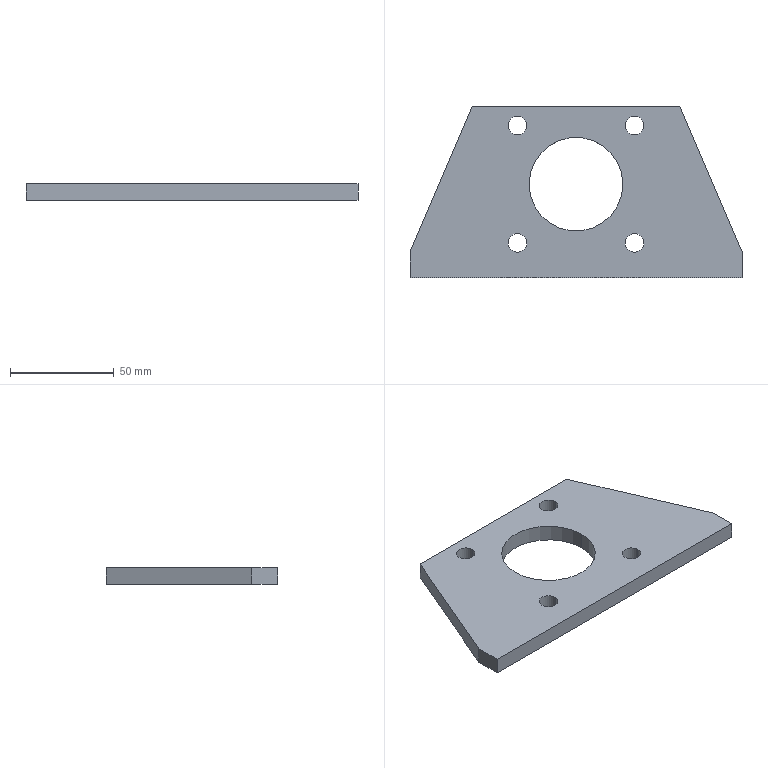Part | SolidWorks | features BaseBody 1, ICE 1 | 1 solid | 18 faces | box 160 x 82.5 x 8 mm | volume 73927 mm3 | cylinder 10 | plane 8 | commonest cylinder face diameters 9 x8 45.2 x2
STEP:
#1=CARTESIAN_POINT('',(22.6,3.75,0.));
#2=VERTEX_POINT('',#1);
#3=CARTESIAN_POINT('',(-22.6,3.75,0.));
#4=VERTEX_POINT('',#3);
#5=CARTESIAN_POINT('',(0.,3.75,0.));
#6=DIRECTION('',(0.,0.,-1.));
#7=DIRECTION('',(1.,0.,0.));
#8=AXIS2_PLACEMENT_3D('',#5,#6,#7);
#9=CIRCLE('',#8,22.6);
#10=EDGE_CURVE('',#2,#4,#9,.T.);
#11=ORIENTED_EDGE('',*,*,#10,.T.);
#12=CARTESIAN_POINT('',(-22.6,3.75,8.));
#13=VERTEX_POINT('',#12);
#14=CARTESIAN_POINT('',(-22.6,3.75,-0.001));
#15=DIRECTION('',(0.,0.,1.));
#16=VECTOR('',#15,1000.);
#17=LINE('',#14,#16);
#18=EDGE_CURVE('',#4,#13,#17,.T.);
#19=ORIENTED_EDGE('',*,*,#18,.T.);
#20=CARTESIAN_POINT('',(22.6,3.75,8.));
#21=VERTEX_POINT('',#20);
#22=CARTESIAN_POINT('',(0.,3.75,8.));
#23=DIRECTION('',(0.,0.,1.));
#24=DIRECTION('',(1.,0.,0.));
#25=AXIS2_PLACEMENT_3D('',#22,#23,#24);
#26=CIRCLE('',#25,22.6);
#27=EDGE_CURVE('',#13,#21,#26,.T.);
#28=ORIENTED_EDGE('',*,*,#27,.T.);
#29=CARTESIAN_POINT('',(22.6,3.75,-0.001));
#30=DIRECTION('',(0.,0.,1.));
#31=VECTOR('',#30,1000.);
#32=LINE('',#29,#31);
#33=EDGE_CURVE('',#2,#21,#32,.T.);
#34=ORIENTED_EDGE('',*,*,#33,.F.);
#35=EDGE_LOOP('',(#11,#19,#28,#34));
#36=FACE_OUTER_BOUND('',#35,.T.);
#37=CARTESIAN_POINT('',(0.,3.75,-0.001));
#38=DIRECTION('',(0.,0.,1.));
#39=DIRECTION('',(1.,0.,0.));
#40=AXIS2_PLACEMENT_3D('',#37,#38,#39);
#41=CYLINDRICAL_SURFACE('',#40,22.6);
#42=ADVANCED_FACE('',(#36),#41,.F.);
#43=CARTESIAN_POINT('',(23.75,-24.5,0.));
#44=VERTEX_POINT('',#43);
#45=CARTESIAN_POINT('',(32.75,-24.5,0.));
#46=VERTEX_POINT('',#45);
#47=CARTESIAN_POINT('',(28.25,-24.5,0.));
#48=DIRECTION('',(0.,0.,1.));
#49=DIRECTION('',(1.,0.,0.));
#50=AXIS2_PLACEMENT_3D('',#47,#48,#49);
#51=CIRCLE('',#50,4.5);
#52=EDGE_CURVE('',#44,#46,#51,.T.);
#53=ORIENTED_EDGE('',*,*,#52,.F.);
#54=CARTESIAN_POINT('',(23.75,-24.5,8.));
#55=VERTEX_POINT('',#54);
#56=CARTESIAN_POINT('',(23.75,-24.5,8.));
#57=DIRECTION('',(0.,0.,1.));
#58=VECTOR('',#57,1000.);
#59=LINE('',#56,#58);
#60=EDGE_CURVE('',#44,#55,#59,.T.);
#61=ORIENTED_EDGE('',*,*,#60,.T.);
#62=CARTESIAN_POINT('',(32.75,-24.5,8.));
#63=VERTEX_POINT('',#62);
#64=CARTESIAN_POINT('',(28.25,-24.5,8.));
#65=DIRECTION('',(0.,0.,1.));
#66=DIRECTION('',(1.,0.,0.));
#67=AXIS2_PLACEMENT_3D('',#64,#65,#66);
#68=CIRCLE('',#67,4.5);
#69=EDGE_CURVE('',#55,#63,#68,.T.);
#70=ORIENTED_EDGE('',*,*,#69,.T.);
#71=CARTESIAN_POINT('',(32.75,-24.5,8.));
#72=DIRECTION('',(0.,0.,1.));
#73=VECTOR('',#72,1000.);
#74=LINE('',#71,#73);
#75=EDGE_CURVE('',#46,#63,#74,.T.);
#76=ORIENTED_EDGE('',*,*,#75,.F.);
#77=EDGE_LOOP('',(#53,#61,#70,#76));
#78=FACE_OUTER_BOUND('',#77,.T.);
#79=CARTESIAN_POINT('',(28.25,-24.5,8.));
#80=DIRECTION('',(0.,0.,1.));
#81=DIRECTION('',(1.,0.,0.));
#82=AXIS2_PLACEMENT_3D('',#79,#80,#81);
#83=CYLINDRICAL_SURFACE('',#82,4.5);
#84=ADVANCED_FACE('',(#78),#83,.F.);
#85=CARTESIAN_POINT('',(23.75,32.,0.));
#86=VERTEX_POINT('',#85);
#87=CARTESIAN_POINT('',(32.75,32.,0.));
#88=VERTEX_POINT('',#87);
#89=CARTESIAN_POINT('',(28.25,32.,0.));
#90=DIRECTION('',(0.,0.,1.));
#91=DIRECTION('',(1.,0.,0.));
#92=AXIS2_PLACEMENT_3D('',#89,#90,#91);
#93=CIRCLE('',#92,4.5);
#94=EDGE_CURVE('',#86,#88,#93,.T.);
#95=ORIENTED_EDGE('',*,*,#94,.F.);
#96=CARTESIAN_POINT('',(23.75,32.,8.));
#97=VERTEX_POINT('',#96);
#98=CARTESIAN_POINT('',(23.75,32.,8.));
#99=DIRECTION('',(0.,0.,1.));
#100=VECTOR('',#99,1000.);
#101=LINE('',#98,#100);
#102=EDGE_CURVE('',#86,#97,#101,.T.);
#103=ORIENTED_EDGE('',*,*,#102,.T.);
#104=CARTESIAN_POINT('',(32.75,32.,8.));
#105=VERTEX_POINT('',#104);
#106=CARTESIAN_POINT('',(28.25,32.,8.));
#107=DIRECTION('',(0.,0.,1.));
#108=DIRECTION('',(1.,0.,0.));
#109=AXIS2_PLACEMENT_3D('',#106,#107,#108);
#110=CIRCLE('',#109,4.5);
#111=EDGE_CURVE('',#97,#105,#110,.T.);
#112=ORIENTED_EDGE('',*,*,#111,.T.);
#113=CARTESIAN_POINT('',(32.75,32.,8.));
#114=DIRECTION('',(0.,0.,1.));
#115=VECTOR('',#114,1000.);
#116=LINE('',#113,#115);
#117=EDGE_CURVE('',#88,#105,#116,.T.);
#118=ORIENTED_EDGE('',*,*,#117,.F.);
#119=EDGE_LOOP('',(#95,#103,#112,#118));
#120=FACE_OUTER_BOUND('',#119,.T.);
#121=CARTESIAN_POINT('',(28.25,32.,8.));
#122=DIRECTION('',(0.,0.,1.));
#123=DIRECTION('',(1.,0.,0.));
#124=AXIS2_PLACEMENT_3D('',#121,#122,#123);
#125=CYLINDRICAL_SURFACE('',#124,4.5);
#126=ADVANCED_FACE('',(#120),#125,.F.);
#127=CARTESIAN_POINT('',(-32.75,-24.5,0.));
#128=VERTEX_POINT('',#127);
#129=CARTESIAN_POINT('',(-23.75,-24.5,0.));
#130=VERTEX_POINT('',#129);
#131=CARTESIAN_POINT('',(-28.25,-24.5,0.));
#132=DIRECTION('',(0.,0.,1.));
#133=DIRECTION('',(1.,0.,0.));
#134=AXIS2_PLACEMENT_3D('',#131,#132,#133);
#135=CIRCLE('',#134,4.5);
#136=EDGE_CURVE('',#128,#130,#135,.T.);
#137=ORIENTED_EDGE('',*,*,#136,.F.);
#138=CARTESIAN_POINT('',(-32.75,-24.5,8.));
#139=VERTEX_POINT('',#138);
#140=CARTESIAN_POINT('',(-32.75,-24.5,8.));
#141=DIRECTION('',(0.,0.,1.));
#142=VECTOR('',#141,1000.);
#143=LINE('',#140,#142);
#144=EDGE_CURVE('',#128,#139,#143,.T.);
#145=ORIENTED_EDGE('',*,*,#144,.T.);
#146=CARTESIAN_POINT('',(-23.75,-24.5,8.));
#147=VERTEX_POINT('',#146);
#148=CARTESIAN_POINT('',(-28.25,-24.5,8.));
#149=DIRECTION('',(0.,0.,1.));
#150=DIRECTION('',(1.,0.,0.));
#151=AXIS2_PLACEMENT_3D('',#148,#149,#150);
#152=CIRCLE('',#151,4.5);
#153=EDGE_CURVE('',#139,#147,#152,.T.);
#154=ORIENTED_EDGE('',*,*,#153,.T.);
#155=CARTESIAN_POINT('',(-23.75,-24.5,8.));
#156=DIRECTION('',(0.,0.,1.));
#157=VECTOR('',#156,1000.);
#158=LINE('',#155,#157);
#159=EDGE_CURVE('',#130,#147,#158,.T.);
#160=ORIENTED_EDGE('',*,*,#159,.F.);
#161=EDGE_LOOP('',(#137,#145,#154,#160));
#162=FACE_OUTER_BOUND('',#161,.T.);
#163=CARTESIAN_POINT('',(-28.25,-24.5,8.));
#164=DIRECTION('',(0.,0.,1.));
#165=DIRECTION('',(1.,0.,0.));
#166=AXIS2_PLACEMENT_3D('',#163,#164,#165);
#167=CYLINDRICAL_SURFACE('',#166,4.5);
#168=ADVANCED_FACE('',(#162),#167,.F.);
#169=CARTESIAN_POINT('',(-32.75,32.,0.));
#170=VERTEX_POINT('',#169);
#171=CARTESIAN_POINT('',(-23.75,32.,0.));
#172=VERTEX_POINT('',#171);
#173=CARTESIAN_POINT('',(-28.25,32.,0.));
#174=DIRECTION('',(0.,0.,1.));
#175=DIRECTION('',(1.,0.,0.));
#176=AXIS2_PLACEMENT_3D('',#173,#174,#175);
#177=CIRCLE('',#176,4.5);
#178=EDGE_CURVE('',#170,#172,#177,.T.);
#179=ORIENTED_EDGE('',*,*,#178,.F.);
#180=CARTESIAN_POINT('',(-32.75,32.,8.));
#181=VERTEX_POINT('',#180);
#182=CARTESIAN_POINT('',(-32.75,32.,8.));
#183=DIRECTION('',(0.,0.,1.));
#184=VECTOR('',#183,1000.);
#185=LINE('',#182,#184);
#186=EDGE_CURVE('',#170,#181,#185,.T.);
#187=ORIENTED_EDGE('',*,*,#186,.T.);
#188=CARTESIAN_POINT('',(-23.75,32.,8.));
#189=VERTEX_POINT('',#188);
#190=CARTESIAN_POINT('',(-28.25,32.,8.));
#191=DIRECTION('',(0.,0.,1.));
#192=DIRECTION('',(1.,0.,0.));
#193=AXIS2_PLACEMENT_3D('',#190,#191,#192);
#194=CIRCLE('',#193,4.5);
#195=EDGE_CURVE('',#181,#189,#194,.T.);
#196=ORIENTED_EDGE('',*,*,#195,.T.);
#197=CARTESIAN_POINT('',(-23.75,32.,8.));
#198=DIRECTION('',(0.,0.,1.));
#199=VECTOR('',#198,1000.);
#200=LINE('',#197,#199);
#201=EDGE_CURVE('',#172,#189,#200,.T.);
#202=ORIENTED_EDGE('',*,*,#201,.F.);
#203=EDGE_LOOP('',(#179,#187,#196,#202));
#204=FACE_OUTER_BOUND('',#203,.T.);
#205=CARTESIAN_POINT('',(-28.25,32.,8.));
#206=DIRECTION('',(0.,0.,1.));
#207=DIRECTION('',(1.,0.,0.));
#208=AXIS2_PLACEMENT_3D('',#205,#206,#207);
#209=CYLINDRICAL_SURFACE('',#208,4.5);
#210=ADVANCED_FACE('',(#204),#209,.F.);
#211=CARTESIAN_POINT('',(-50.,41.25,8.));
#212=VERTEX_POINT('',#211);
#213=CARTESIAN_POINT('',(-50.,41.25,0.));
#214=VERTEX_POINT('',#213);
#215=CARTESIAN_POINT('',(-50.,41.25,10.));
#216=DIRECTION('',(0.,0.,-1.));
#217=VECTOR('',#216,1000.);
#218=LINE('',#215,#217);
#219=EDGE_CURVE('',#212,#214,#218,.T.);
#220=ORIENTED_EDGE('',*,*,#219,.T.);
#221=CARTESIAN_POINT('',(-80.,-28.75,0.));
#222=VERTEX_POINT('',#221);
#223=CARTESIAN_POINT('',(-50.,41.25,0.));
#224=DIRECTION('',(0.3939,0.9191,0.));
#225=VECTOR('',#224,1000.);
#226=LINE('',#223,#225);
#227=EDGE_CURVE('',#222,#214,#226,.T.);
#228=ORIENTED_EDGE('',*,*,#227,.F.);
#229=CARTESIAN_POINT('',(-80.,-28.75,8.));
#230=VERTEX_POINT('',#229);
#231=CARTESIAN_POINT('',(-80.,-28.75,10.));
#232=DIRECTION('',(0.,0.,-1.));
#233=VECTOR('',#232,1000.);
#234=LINE('',#231,#233);
#235=EDGE_CURVE('',#230,#222,#234,.T.);
#236=ORIENTED_EDGE('',*,*,#235,.F.);
#237=CARTESIAN_POINT('',(-57.177,24.504,8.));
#238=DIRECTION('',(-0.3939,-0.9191,0.));
#239=VECTOR('',#238,1000.);
#240=LINE('',#237,#239);
#241=EDGE_CURVE('',#212,#230,#240,.T.);
#242=ORIENTED_EDGE('',*,*,#241,.F.);
#243=EDGE_LOOP('',(#220,#228,#236,#242));
#244=FACE_OUTER_BOUND('',#243,.T.);
#245=CARTESIAN_POINT('',(-50.,41.25,10.));
#246=DIRECTION('',(-0.9191,0.3939,0.));
#247=DIRECTION('',(0.,0.,1.));
#248=AXIS2_PLACEMENT_3D('',#245,#246,#247);
#249=PLANE('',#248);
#250=ADVANCED_FACE('',(#244),#249,.T.);
#251=CARTESIAN_POINT('',(50.,41.25,8.));
#252=VERTEX_POINT('',#251);
#253=CARTESIAN_POINT('',(80.,-28.75,8.));
#254=VERTEX_POINT('',#253);
#255=CARTESIAN_POINT('',(57.177,24.504,8.));
#256=DIRECTION('',(0.3939,-0.9191,0.));
#257=VECTOR('',#256,1000.);
#258=LINE('',#255,#257);
#259=EDGE_CURVE('',#252,#254,#258,.T.);
#260=ORIENTED_EDGE('',*,*,#259,.T.);
#261=CARTESIAN_POINT('',(80.,-28.75,0.));
#262=VERTEX_POINT('',#261);
#263=CARTESIAN_POINT('',(80.,-28.75,10.));
#264=DIRECTION('',(0.,0.,-1.));
#265=VECTOR('',#264,1000.);
#266=LINE('',#263,#265);
#267=EDGE_CURVE('',#254,#262,#266,.T.);
#268=ORIENTED_EDGE('',*,*,#267,.T.);
#269=CARTESIAN_POINT('',(50.,41.25,0.));
#270=VERTEX_POINT('',#269);
#271=CARTESIAN_POINT('',(50.,41.25,0.));
#272=DIRECTION('',(-0.3939,0.9191,0.));
#273=VECTOR('',#272,1000.);
#274=LINE('',#271,#273);
#275=EDGE_CURVE('',#262,#270,#274,.T.);
#276=ORIENTED_EDGE('',*,*,#275,.T.);
#277=CARTESIAN_POINT('',(50.,41.25,10.));
#278=DIRECTION('',(0.,0.,-1.));
#279=VECTOR('',#278,1000.);
#280=LINE('',#277,#279);
#281=EDGE_CURVE('',#252,#270,#280,.T.);
#282=ORIENTED_EDGE('',*,*,#281,.F.);
#283=EDGE_LOOP('',(#260,#268,#276,#282));
#284=FACE_OUTER_BOUND('',#283,.T.);
#285=CARTESIAN_POINT('',(50.,41.25,10.));
#286=DIRECTION('',(-0.9191,-0.3939,0.));
#287=DIRECTION('',(-0.3939,0.9191,0.));
#288=AXIS2_PLACEMENT_3D('',#285,#286,#287);
#289=PLANE('',#288);
#290=ADVANCED_FACE('',(#284),#289,.F.);
#291=CARTESIAN_POINT('',(-80.,-41.25,0.));
#292=VERTEX_POINT('',#291);
#293=CARTESIAN_POINT('',(80.,-41.25,0.));
#294=VERTEX_POINT('',#293);
#295=CARTESIAN_POINT('',(-80.,-41.25,0.));
#296=DIRECTION('',(1.,0.,0.));
#297=VECTOR('',#296,1000.);
#298=LINE('',#295,#297);
#299=EDGE_CURVE('',#292,#294,#298,.T.);
#300=ORIENTED_EDGE('',*,*,#299,.T.);
#301=CARTESIAN_POINT('',(80.,-41.25,8.));
#302=VERTEX_POINT('',#301);
#303=CARTESIAN_POINT('',(80.,-41.25,8.));
#304=DIRECTION('',(0.,0.,-1.));
#305=VECTOR('',#304,1000.);
#306=LINE('',#303,#305);
#307=EDGE_CURVE('',#302,#294,#306,.T.);
#308=ORIENTED_EDGE('',*,*,#307,.F.);
#309=CARTESIAN_POINT('',(-80.,-41.25,8.));
#310=VERTEX_POINT('',#309);
#311=CARTESIAN_POINT('',(-80.,-41.25,8.));
#312=DIRECTION('',(1.,0.,0.));
#313=VECTOR('',#312,1000.);
#314=LINE('',#311,#313);
#315=EDGE_CURVE('',#310,#302,#314,.T.);
#316=ORIENTED_EDGE('',*,*,#315,.F.);
#317=CARTESIAN_POINT('',(-80.,-41.25,8.));
#318=DIRECTION('',(0.,0.,-1.));
#319=VECTOR('',#318,1000.);
#320=LINE('',#317,#319);
#321=EDGE_CURVE('',#310,#292,#320,.T.);
#322=ORIENTED_EDGE('',*,*,#321,.T.);
#323=EDGE_LOOP('',(#300,#308,#316,#322));
#324=FACE_OUTER_BOUND('',#323,.T.);
#325=CARTESIAN_POINT('',(-80.,-41.25,8.));
#326=DIRECTION('',(0.,1.,0.));
#327=DIRECTION('',(1.,0.,0.));
#328=AXIS2_PLACEMENT_3D('',#325,#326,#327);
#329=PLANE('',#328);
#330=ADVANCED_FACE('',(#324),#329,.F.);
#331=CARTESIAN_POINT('',(80.,41.25,0.));
#332=DIRECTION('',(0.,1.,0.));
#333=VECTOR('',#332,1000.);
#334=LINE('',#331,#333);
#335=EDGE_CURVE('',#294,#262,#334,.T.);
#336=ORIENTED_EDGE('',*,*,#335,.T.);
#337=ORIENTED_EDGE('',*,*,#267,.F.);
#338=CARTESIAN_POINT('',(80.,41.25,8.));
#339=DIRECTION('',(0.,1.,0.));
#340=VECTOR('',#339,1000.);
#341=LINE('',#338,#340);
#342=EDGE_CURVE('',#302,#254,#341,.T.);
#343=ORIENTED_EDGE('',*,*,#342,.F.);
#344=ORIENTED_EDGE('',*,*,#307,.T.);
#345=EDGE_LOOP('',(#336,#337,#343,#344));
#346=FACE_OUTER_BOUND('',#345,.T.);
#347=CARTESIAN_POINT('',(80.,41.25,8.));
#348=DIRECTION('',(-1.,0.,0.));
#349=DIRECTION('',(0.,0.,1.));
#350=AXIS2_PLACEMENT_3D('',#347,#348,#349);
#351=PLANE('',#350);
#352=ADVANCED_FACE('',(#346),#351,.F.);
#353=ORIENTED_EDGE('',*,*,#10,.F.);
#354=CARTESIAN_POINT('',(0.,3.75,0.));
#355=DIRECTION('',(0.,0.,-1.));
#356=DIRECTION('',(1.,0.,0.));
#357=AXIS2_PLACEMENT_3D('',#354,#355,#356);
#358=CIRCLE('',#357,22.6);
#359=EDGE_CURVE('',#4,#2,#358,.T.);
#360=ORIENTED_EDGE('',*,*,#359,.F.);
#361=EDGE_LOOP('',(#353,#360));
#362=FACE_BOUND('',#361,.T.);
#363=CARTESIAN_POINT('',(28.25,-24.5,0.));
#364=DIRECTION('',(0.,0.,1.));
#365=DIRECTION('',(1.,0.,0.));
#366=AXIS2_PLACEMENT_3D('',#363,#364,#365);
#367=CIRCLE('',#366,4.5);
#368=EDGE_CURVE('',#46,#44,#367,.T.);
#369=ORIENTED_EDGE('',*,*,#368,.T.);
#370=ORIENTED_EDGE('',*,*,#52,.T.);
#371=EDGE_LOOP('',(#369,#370));
#372=FACE_BOUND('',#371,.T.);
#373=CARTESIAN_POINT('',(28.25,32.,0.));
#374=DIRECTION('',(0.,0.,1.));
#375=DIRECTION('',(1.,0.,0.));
#376=AXIS2_PLACEMENT_3D('',#373,#374,#375);
#377=CIRCLE('',#376,4.5);
#378=EDGE_CURVE('',#88,#86,#377,.T.);
#379=ORIENTED_EDGE('',*,*,#378,.T.);
#380=ORIENTED_EDGE('',*,*,#94,.T.);
#381=EDGE_LOOP('',(#379,#380));
#382=FACE_BOUND('',#381,.T.);
#383=CARTESIAN_POINT('',(-28.25,-24.5,0.));
#384=DIRECTION('',(0.,0.,1.));
#385=DIRECTION('',(1.,0.,0.));
#386=AXIS2_PLACEMENT_3D('',#383,#384,#385);
#387=CIRCLE('',#386,4.5);
#388=EDGE_CURVE('',#130,#128,#387,.T.);
#389=ORIENTED_EDGE('',*,*,#388,.T.);
#390=ORIENTED_EDGE('',*,*,#136,.T.);
#391=EDGE_LOOP('',(#389,#390));
#392=FACE_BOUND('',#391,.T.);
#393=CARTESIAN_POINT('',(-28.25,32.,0.));
#394=DIRECTION('',(0.,0.,1.));
#395=DIRECTION('',(1.,0.,0.));
#396=AXIS2_PLACEMENT_3D('',#393,#394,#395);
#397=CIRCLE('',#396,4.5);
#398=EDGE_CURVE('',#172,#170,#397,.T.);
#399=ORIENTED_EDGE('',*,*,#398,.T.);
#400=ORIENTED_EDGE('',*,*,#178,.T.);
#401=EDGE_LOOP('',(#399,#400));
#402=FACE_BOUND('',#401,.T.);
#403=ORIENTED_EDGE('',*,*,#227,.T.);
#404=CARTESIAN_POINT('',(-80.,41.25,0.));
#405=DIRECTION('',(-1.,0.,0.));
#406=VECTOR('',#405,1000.);
#407=LINE('',#404,#406);
#408=EDGE_CURVE('',#270,#214,#407,.T.);
#409=ORIENTED_EDGE('',*,*,#408,.F.);
#410=ORIENTED_EDGE('',*,*,#275,.F.);
#411=ORIENTED_EDGE('',*,*,#335,.F.);
#412=ORIENTED_EDGE('',*,*,#299,.F.);
#413=CARTESIAN_POINT('',(-80.,41.25,0.));
#414=DIRECTION('',(0.,-1.,0.));
#415=VECTOR('',#414,1000.);
#416=LINE('',#413,#415);
#417=EDGE_CURVE('',#222,#292,#416,.T.);
#418=ORIENTED_EDGE('',*,*,#417,.F.);
#419=EDGE_LOOP('',(#403,#409,#410,#411,#412,#418));
#420=FACE_OUTER_BOUND('',#419,.T.);
#421=CARTESIAN_POINT('',(0.,0.,0.));
#422=DIRECTION('',(0.,0.,1.));
#423=DIRECTION('',(1.,0.,0.));
#424=AXIS2_PLACEMENT_3D('',#421,#422,#423);
#425=PLANE('',#424);
#426=ADVANCED_FACE('',(#362,#372,#382,#392,#402,#420),#425,.F.);
#427=CARTESIAN_POINT('',(0.,3.75,8.));
#428=DIRECTION('',(0.,0.,1.));
#429=DIRECTION('',(1.,0.,0.));
#430=AXIS2_PLACEMENT_3D('',#427,#428,#429);
#431=CIRCLE('',#430,22.6);
#432=EDGE_CURVE('',#21,#13,#431,.T.);
#433=ORIENTED_EDGE('',*,*,#432,.F.);
#434=ORIENTED_EDGE('',*,*,#27,.F.);
#435=EDGE_LOOP('',(#433,#434));
#436=FACE_BOUND('',#435,.T.);
#437=CARTESIAN_POINT('',(-28.25,32.,8.));
#438=DIRECTION('',(0.,0.,1.));
#439=DIRECTION('',(1.,0.,0.));
#440=AXIS2_PLACEMENT_3D('',#437,#438,#439);
#441=CIRCLE('',#440,4.5);
#442=EDGE_CURVE('',#189,#181,#441,.T.);
#443=ORIENTED_EDGE('',*,*,#442,.F.);
#444=ORIENTED_EDGE('',*,*,#195,.F.);
#445=EDGE_LOOP('',(#443,#444));
#446=FACE_BOUND('',#445,.T.);
#447=CARTESIAN_POINT('',(-28.25,-24.5,8.));
#448=DIRECTION('',(0.,0.,1.));
#449=DIRECTION('',(1.,0.,0.));
#450=AXIS2_PLACEMENT_3D('',#447,#448,#449);
#451=CIRCLE('',#450,4.5);
#452=EDGE_CURVE('',#147,#139,#451,.T.);
#453=ORIENTED_EDGE('',*,*,#452,.F.);
#454=ORIENTED_EDGE('',*,*,#153,.F.);
#455=EDGE_LOOP('',(#453,#454));
#456=FACE_BOUND('',#455,.T.);
#457=CARTESIAN_POINT('',(28.25,32.,8.));
#458=DIRECTION('',(0.,0.,1.));
#459=DIRECTION('',(1.,0.,0.));
#460=AXIS2_PLACEMENT_3D('',#457,#458,#459);
#461=CIRCLE('',#460,4.5);
#462=EDGE_CURVE('',#105,#97,#461,.T.);
#463=ORIENTED_EDGE('',*,*,#462,.F.);
#464=ORIENTED_EDGE('',*,*,#111,.F.);
#465=EDGE_LOOP('',(#463,#464));
#466=FACE_BOUND('',#465,.T.);
#467=CARTESIAN_POINT('',(28.25,-24.5,8.));
#468=DIRECTION('',(0.,0.,1.));
#469=DIRECTION('',(1.,0.,0.));
#470=AXIS2_PLACEMENT_3D('',#467,#468,#469);
#471=CIRCLE('',#470,4.5);
#472=EDGE_CURVE('',#63,#55,#471,.T.);
#473=ORIENTED_EDGE('',*,*,#472,.F.);
#474=ORIENTED_EDGE('',*,*,#69,.F.);
#475=EDGE_LOOP('',(#473,#474));
#476=FACE_BOUND('',#475,.T.);
#477=CARTESIAN_POINT('',(-80.,41.25,8.));
#478=DIRECTION('',(-1.,0.,0.));
#479=VECTOR('',#478,1000.);
#480=LINE('',#477,#479);
#481=EDGE_CURVE('',#252,#212,#480,.T.);
#482=ORIENTED_EDGE('',*,*,#481,.T.);
#483=ORIENTED_EDGE('',*,*,#241,.T.);
#484=CARTESIAN_POINT('',(-80.,41.25,8.));
#485=DIRECTION('',(0.,-1.,0.));
#486=VECTOR('',#485,1000.);
#487=LINE('',#484,#486);
#488=EDGE_CURVE('',#230,#310,#487,.T.);
#489=ORIENTED_EDGE('',*,*,#488,.T.);
#490=ORIENTED_EDGE('',*,*,#315,.T.);
#491=ORIENTED_EDGE('',*,*,#342,.T.);
#492=ORIENTED_EDGE('',*,*,#259,.F.);
#493=EDGE_LOOP('',(#482,#483,#489,#490,#491,#492));
#494=FACE_OUTER_BOUND('',#493,.T.);
#495=CARTESIAN_POINT('',(0.,0.,8.));
#496=DIRECTION('',(0.,0.,1.));
#497=DIRECTION('',(1.,0.,0.));
#498=AXIS2_PLACEMENT_3D('',#495,#496,#497);
#499=PLANE('',#498);
#500=ADVANCED_FACE('',(#436,#446,#456,#466,#476,#494),#499,.T.);
#501=ORIENTED_EDGE('',*,*,#235,.T.);
#502=ORIENTED_EDGE('',*,*,#417,.T.);
#503=ORIENTED_EDGE('',*,*,#321,.F.);
#504=ORIENTED_EDGE('',*,*,#488,.F.);
#505=EDGE_LOOP('',(#501,#502,#503,#504));
#506=FACE_OUTER_BOUND('',#505,.T.);
#507=CARTESIAN_POINT('',(-80.,41.25,8.));
#508=DIRECTION('',(1.,0.,0.));
#509=DIRECTION('',(0.,1.,0.));
#510=AXIS2_PLACEMENT_3D('',#507,#508,#509);
#511=PLANE('',#510);
#512=ADVANCED_FACE('',(#506),#511,.F.);
#513=ORIENTED_EDGE('',*,*,#219,.F.);
#514=ORIENTED_EDGE('',*,*,#481,.F.);
#515=ORIENTED_EDGE('',*,*,#281,.T.);
#516=ORIENTED_EDGE('',*,*,#408,.T.);
#517=EDGE_LOOP('',(#513,#514,#515,#516));
#518=FACE_OUTER_BOUND('',#517,.T.);
#519=CARTESIAN_POINT('',(-80.,41.25,8.));
#520=DIRECTION('',(0.,-1.,0.));
#521=DIRECTION('',(0.,0.,-1.));
#522=AXIS2_PLACEMENT_3D('',#519,#520,#521);
#523=PLANE('',#522);
#524=ADVANCED_FACE('',(#518),#523,.F.);
#525=ORIENTED_EDGE('',*,*,#186,.F.);
#526=ORIENTED_EDGE('',*,*,#398,.F.);
#527=ORIENTED_EDGE('',*,*,#201,.T.);
#528=ORIENTED_EDGE('',*,*,#442,.T.);
#529=EDGE_LOOP('',(#525,#526,#527,#528));
#530=FACE_OUTER_BOUND('',#529,.T.);
#531=CARTESIAN_POINT('',(-28.25,32.,8.));
#532=DIRECTION('',(0.,0.,1.));
#533=DIRECTION('',(1.,0.,0.));
#534=AXIS2_PLACEMENT_3D('',#531,#532,#533);
#535=CYLINDRICAL_SURFACE('',#534,4.5);
#536=ADVANCED_FACE('',(#530),#535,.F.);
#537=ORIENTED_EDGE('',*,*,#144,.F.);
#538=ORIENTED_EDGE('',*,*,#388,.F.);
#539=ORIENTED_EDGE('',*,*,#159,.T.);
#540=ORIENTED_EDGE('',*,*,#452,.T.);
#541=EDGE_LOOP('',(#537,#538,#539,#540));
#542=FACE_OUTER_BOUND('',#541,.T.);
#543=CARTESIAN_POINT('',(-28.25,-24.5,8.));
#544=DIRECTION('',(0.,0.,1.));
#545=DIRECTION('',(1.,0.,0.));
#546=AXIS2_PLACEMENT_3D('',#543,#544,#545);
#547=CYLINDRICAL_SURFACE('',#546,4.5);
#548=ADVANCED_FACE('',(#542),#547,.F.);
#549=ORIENTED_EDGE('',*,*,#102,.F.);
#550=ORIENTED_EDGE('',*,*,#378,.F.);
#551=ORIENTED_EDGE('',*,*,#117,.T.);
#552=ORIENTED_EDGE('',*,*,#462,.T.);
#553=EDGE_LOOP('',(#549,#550,#551,#552));
#554=FACE_OUTER_BOUND('',#553,.T.);
#555=CARTESIAN_POINT('',(28.25,32.,8.));
#556=DIRECTION('',(0.,0.,1.));
#557=DIRECTION('',(1.,0.,0.));
#558=AXIS2_PLACEMENT_3D('',#555,#556,#557);
#559=CYLINDRICAL_SURFACE('',#558,4.5);
#560=ADVANCED_FACE('',(#554),#559,.F.);
#561=ORIENTED_EDGE('',*,*,#60,.F.);
#562=ORIENTED_EDGE('',*,*,#368,.F.);
#563=ORIENTED_EDGE('',*,*,#75,.T.);
#564=ORIENTED_EDGE('',*,*,#472,.T.);
#565=EDGE_LOOP('',(#561,#562,#563,#564));
#566=FACE_OUTER_BOUND('',#565,.T.);
#567=CARTESIAN_POINT('',(28.25,-24.5,8.));
#568=DIRECTION('',(0.,0.,1.));
#569=DIRECTION('',(1.,0.,0.));
#570=AXIS2_PLACEMENT_3D('',#567,#568,#569);
#571=CYLINDRICAL_SURFACE('',#570,4.5);
#572=ADVANCED_FACE('',(#566),#571,.F.);
#573=ORIENTED_EDGE('',*,*,#18,.F.);
#574=ORIENTED_EDGE('',*,*,#359,.T.);
#575=ORIENTED_EDGE('',*,*,#33,.T.);
#576=ORIENTED_EDGE('',*,*,#432,.T.);
#577=EDGE_LOOP('',(#573,#574,#575,#576));
#578=FACE_OUTER_BOUND('',#577,.T.);
#579=CARTESIAN_POINT('',(0.,3.75,-0.001));
#580=DIRECTION('',(0.,0.,1.));
#581=DIRECTION('',(1.,0.,0.));
#582=AXIS2_PLACEMENT_3D('',#579,#580,#581);
#583=CYLINDRICAL_SURFACE('',#582,22.6);
#584=ADVANCED_FACE('',(#578),#583,.F.);
#585=CLOSED_SHELL('',(#42,#84,#126,#168,#210,#250,#290,#330,#352,#426,#500,#512,#524,#536,#548,#560,#572,#584));
#586=MANIFOLD_SOLID_BREP('',#585);
#587=CARTESIAN_POINT('',(0.,0.,0.));
#588=DIRECTION('',(0.,0.,1.));
#589=DIRECTION('',(1.,0.,0.));
#590=AXIS2_PLACEMENT_3D('',#587,#588,#589);
#591=(LENGTH_UNIT()NAMED_UNIT(*)SI_UNIT(.MILLI.,.METRE.));
#592=UNCERTAINTY_MEASURE_WITH_UNIT(LENGTH_MEASURE(0.00001),#591,'','');
#593=(NAMED_UNIT(*)PLANE_ANGLE_UNIT()SI_UNIT($,.RADIAN.));
#594=(NAMED_UNIT(*)SI_UNIT($,.STERADIAN.)SOLID_ANGLE_UNIT());
#595=(GEOMETRIC_REPRESENTATION_CONTEXT(3)GLOBAL_UNCERTAINTY_ASSIGNED_CONTEXT((#592))GLOBAL_UNIT_ASSIGNED_CONTEXT((#591,#593,#594))REPRESENTATION_CONTEXT('',''));
#596=ADVANCED_BREP_SHAPE_REPRESENTATION('',(#586,#590),#595);